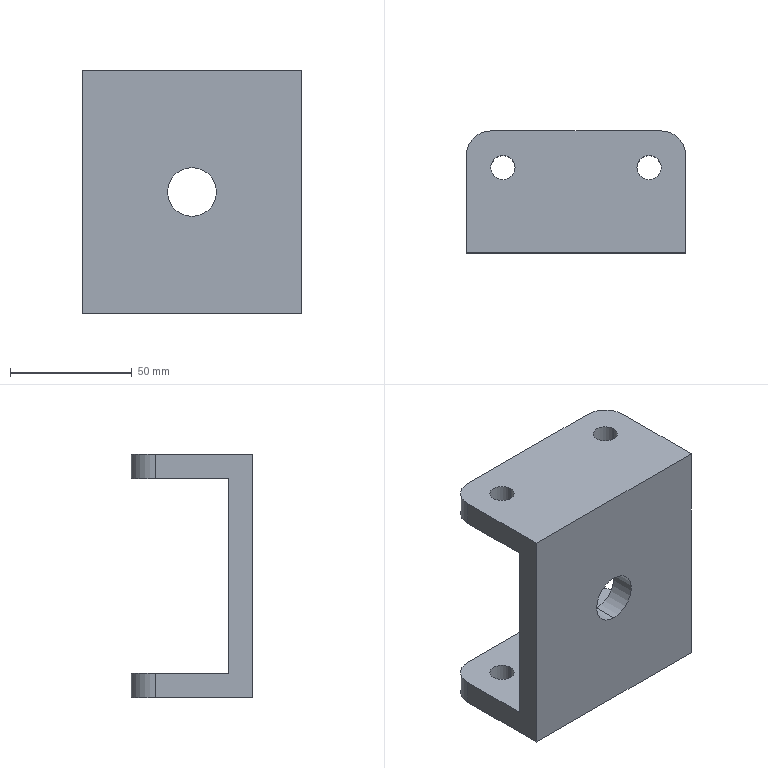Part | SolidWorks | features ICE 4, MoveFace 4, Extrusion 1, Fillet 1 | 1 solid | 24 faces | box 90 x 50 x 100 mm | volume 154858 mm3 | cylinder 14 | plane 10 | commonest cylinder face diameters 10 x8 20 x6
STEP:
#1=CARTESIAN_POINT('',(-5.,0.,-35.));
#2=VERTEX_POINT('',#1);
#3=CARTESIAN_POINT('',(-5.,0.,-15.));
#4=VERTEX_POINT('',#3);
#5=CARTESIAN_POINT('',(-5.,0.,-25.));
#6=DIRECTION('',(0.,1.,0.));
#7=DIRECTION('',(0.,0.,1.));
#8=AXIS2_PLACEMENT_3D('',#5,#6,#7);
#9=CIRCLE('',#8,10.);
#10=EDGE_CURVE('',#2,#4,#9,.T.);
#11=ORIENTED_EDGE('',*,*,#10,.F.);
#12=CARTESIAN_POINT('',(-5.,10.,-35.));
#13=VERTEX_POINT('',#12);
#14=CARTESIAN_POINT('',(-5.,0.,-35.));
#15=DIRECTION('',(0.,1.,0.));
#16=VECTOR('',#15,1000.);
#17=LINE('',#14,#16);
#18=EDGE_CURVE('',#2,#13,#17,.T.);
#19=ORIENTED_EDGE('',*,*,#18,.T.);
#20=CARTESIAN_POINT('',(-5.,10.,-15.));
#21=VERTEX_POINT('',#20);
#22=CARTESIAN_POINT('',(-5.,10.,-25.));
#23=DIRECTION('',(0.,1.,0.));
#24=DIRECTION('',(0.,0.,1.));
#25=AXIS2_PLACEMENT_3D('',#22,#23,#24);
#26=CIRCLE('',#25,10.);
#27=EDGE_CURVE('',#13,#21,#26,.T.);
#28=ORIENTED_EDGE('',*,*,#27,.T.);
#29=CARTESIAN_POINT('',(-5.,0.,-15.));
#30=DIRECTION('',(0.,1.,0.));
#31=VECTOR('',#30,1000.);
#32=LINE('',#29,#31);
#33=EDGE_CURVE('',#4,#21,#32,.T.);
#34=ORIENTED_EDGE('',*,*,#33,.F.);
#35=EDGE_LOOP('',(#11,#19,#28,#34));
#36=FACE_OUTER_BOUND('',#35,.T.);
#37=CARTESIAN_POINT('',(-5.,0.,-25.));
#38=DIRECTION('',(0.,1.,0.));
#39=DIRECTION('',(0.,0.,1.));
#40=AXIS2_PLACEMENT_3D('',#37,#38,#39);
#41=CYLINDRICAL_SURFACE('',#40,10.);
#42=ADVANCED_FACE('',(#36),#41,.F.);
#43=CARTESIAN_POINT('',(20.,35.,-75.));
#44=VERTEX_POINT('',#43);
#45=CARTESIAN_POINT('',(30.,35.,-75.));
#46=VERTEX_POINT('',#45);
#47=CARTESIAN_POINT('',(25.,35.,-75.));
#48=DIRECTION('',(0.,0.,1.));
#49=DIRECTION('',(1.,0.,0.));
#50=AXIS2_PLACEMENT_3D('',#47,#48,#49);
#51=CIRCLE('',#50,5.);
#52=EDGE_CURVE('',#44,#46,#51,.T.);
#53=ORIENTED_EDGE('',*,*,#52,.F.);
#54=CARTESIAN_POINT('',(20.,35.,-65.));
#55=VERTEX_POINT('',#54);
#56=CARTESIAN_POINT('',(20.,35.,-25.));
#57=DIRECTION('',(0.,0.,1.));
#58=VECTOR('',#57,1000.);
#59=LINE('',#56,#58);
#60=EDGE_CURVE('',#44,#55,#59,.T.);
#61=ORIENTED_EDGE('',*,*,#60,.T.);
#62=CARTESIAN_POINT('',(30.,35.,-65.));
#63=VERTEX_POINT('',#62);
#64=CARTESIAN_POINT('',(25.,35.,-65.));
#65=DIRECTION('',(0.,0.,-1.));
#66=DIRECTION('',(0.,1.,0.));
#67=AXIS2_PLACEMENT_3D('',#64,#65,#66);
#68=CIRCLE('',#67,5.);
#69=EDGE_CURVE('',#63,#55,#68,.T.);
#70=ORIENTED_EDGE('',*,*,#69,.F.);
#71=CARTESIAN_POINT('',(30.,35.,-25.));
#72=DIRECTION('',(0.,0.,1.));
#73=VECTOR('',#72,1000.);
#74=LINE('',#71,#73);
#75=EDGE_CURVE('',#46,#63,#74,.T.);
#76=ORIENTED_EDGE('',*,*,#75,.F.);
#77=EDGE_LOOP('',(#53,#61,#70,#76));
#78=FACE_OUTER_BOUND('',#77,.T.);
#79=CARTESIAN_POINT('',(25.,35.,-25.));
#80=DIRECTION('',(0.,0.,1.));
#81=DIRECTION('',(1.,0.,0.));
#82=AXIS2_PLACEMENT_3D('',#79,#80,#81);
#83=CYLINDRICAL_SURFACE('',#82,5.);
#84=ADVANCED_FACE('',(#78),#83,.F.);
#85=CARTESIAN_POINT('',(-40.,35.,-75.));
#86=VERTEX_POINT('',#85);
#87=CARTESIAN_POINT('',(-30.,35.,-75.));
#88=VERTEX_POINT('',#87);
#89=CARTESIAN_POINT('',(-35.,35.,-75.));
#90=DIRECTION('',(0.,0.,1.));
#91=DIRECTION('',(1.,0.,0.));
#92=AXIS2_PLACEMENT_3D('',#89,#90,#91);
#93=CIRCLE('',#92,5.);
#94=EDGE_CURVE('',#86,#88,#93,.T.);
#95=ORIENTED_EDGE('',*,*,#94,.F.);
#96=CARTESIAN_POINT('',(-40.,35.,-65.));
#97=VERTEX_POINT('',#96);
#98=CARTESIAN_POINT('',(-40.,35.,-25.));
#99=DIRECTION('',(0.,0.,1.));
#100=VECTOR('',#99,1000.);
#101=LINE('',#98,#100);
#102=EDGE_CURVE('',#86,#97,#101,.T.);
#103=ORIENTED_EDGE('',*,*,#102,.T.);
#104=CARTESIAN_POINT('',(-30.,35.,-65.));
#105=VERTEX_POINT('',#104);
#106=CARTESIAN_POINT('',(-35.,35.,-65.));
#107=DIRECTION('',(0.,0.,-1.));
#108=DIRECTION('',(0.,1.,0.));
#109=AXIS2_PLACEMENT_3D('',#106,#107,#108);
#110=CIRCLE('',#109,5.);
#111=EDGE_CURVE('',#105,#97,#110,.T.);
#112=ORIENTED_EDGE('',*,*,#111,.F.);
#113=CARTESIAN_POINT('',(-30.,35.,-25.));
#114=DIRECTION('',(0.,0.,1.));
#115=VECTOR('',#114,1000.);
#116=LINE('',#113,#115);
#117=EDGE_CURVE('',#88,#105,#116,.T.);
#118=ORIENTED_EDGE('',*,*,#117,.F.);
#119=EDGE_LOOP('',(#95,#103,#112,#118));
#120=FACE_OUTER_BOUND('',#119,.T.);
#121=CARTESIAN_POINT('',(-35.,35.,-25.));
#122=DIRECTION('',(0.,0.,1.));
#123=DIRECTION('',(1.,0.,0.));
#124=AXIS2_PLACEMENT_3D('',#121,#122,#123);
#125=CYLINDRICAL_SURFACE('',#124,5.);
#126=ADVANCED_FACE('',(#120),#125,.F.);
#127=CARTESIAN_POINT('',(20.,35.,15.));
#128=VERTEX_POINT('',#127);
#129=CARTESIAN_POINT('',(30.,35.,15.));
#130=VERTEX_POINT('',#129);
#131=CARTESIAN_POINT('',(25.,35.,15.));
#132=DIRECTION('',(0.,0.,1.));
#133=DIRECTION('',(0.,-1.,0.));
#134=AXIS2_PLACEMENT_3D('',#131,#132,#133);
#135=CIRCLE('',#134,5.);
#136=EDGE_CURVE('',#128,#130,#135,.T.);
#137=ORIENTED_EDGE('',*,*,#136,.F.);
#138=CARTESIAN_POINT('',(20.,35.,25.));
#139=VERTEX_POINT('',#138);
#140=CARTESIAN_POINT('',(20.,35.,-25.));
#141=DIRECTION('',(0.,0.,1.));
#142=VECTOR('',#141,1000.);
#143=LINE('',#140,#142);
#144=EDGE_CURVE('',#128,#139,#143,.T.);
#145=ORIENTED_EDGE('',*,*,#144,.T.);
#146=CARTESIAN_POINT('',(30.,35.,25.));
#147=VERTEX_POINT('',#146);
#148=CARTESIAN_POINT('',(25.,35.,25.));
#149=DIRECTION('',(0.,0.,1.));
#150=DIRECTION('',(1.,0.,0.));
#151=AXIS2_PLACEMENT_3D('',#148,#149,#150);
#152=CIRCLE('',#151,5.);
#153=EDGE_CURVE('',#139,#147,#152,.T.);
#154=ORIENTED_EDGE('',*,*,#153,.T.);
#155=CARTESIAN_POINT('',(30.,35.,-25.));
#156=DIRECTION('',(0.,0.,1.));
#157=VECTOR('',#156,1000.);
#158=LINE('',#155,#157);
#159=EDGE_CURVE('',#130,#147,#158,.T.);
#160=ORIENTED_EDGE('',*,*,#159,.F.);
#161=EDGE_LOOP('',(#137,#145,#154,#160));
#162=FACE_OUTER_BOUND('',#161,.T.);
#163=CARTESIAN_POINT('',(25.,35.,-25.));
#164=DIRECTION('',(0.,0.,1.));
#165=DIRECTION('',(1.,0.,0.));
#166=AXIS2_PLACEMENT_3D('',#163,#164,#165);
#167=CYLINDRICAL_SURFACE('',#166,5.);
#168=ADVANCED_FACE('',(#162),#167,.F.);
#169=CARTESIAN_POINT('',(-40.,35.,15.));
#170=VERTEX_POINT('',#169);
#171=CARTESIAN_POINT('',(-30.,35.,15.));
#172=VERTEX_POINT('',#171);
#173=CARTESIAN_POINT('',(-35.,35.,15.));
#174=DIRECTION('',(0.,0.,1.));
#175=DIRECTION('',(0.,-1.,0.));
#176=AXIS2_PLACEMENT_3D('',#173,#174,#175);
#177=CIRCLE('',#176,5.);
#178=EDGE_CURVE('',#170,#172,#177,.T.);
#179=ORIENTED_EDGE('',*,*,#178,.F.);
#180=CARTESIAN_POINT('',(-40.,35.,25.));
#181=VERTEX_POINT('',#180);
#182=CARTESIAN_POINT('',(-40.,35.,-25.));
#183=DIRECTION('',(0.,0.,1.));
#184=VECTOR('',#183,1000.);
#185=LINE('',#182,#184);
#186=EDGE_CURVE('',#170,#181,#185,.T.);
#187=ORIENTED_EDGE('',*,*,#186,.T.);
#188=CARTESIAN_POINT('',(-30.,35.,25.));
#189=VERTEX_POINT('',#188);
#190=CARTESIAN_POINT('',(-35.,35.,25.));
#191=DIRECTION('',(0.,0.,1.));
#192=DIRECTION('',(1.,0.,0.));
#193=AXIS2_PLACEMENT_3D('',#190,#191,#192);
#194=CIRCLE('',#193,5.);
#195=EDGE_CURVE('',#181,#189,#194,.T.);
#196=ORIENTED_EDGE('',*,*,#195,.T.);
#197=CARTESIAN_POINT('',(-30.,35.,-25.));
#198=DIRECTION('',(0.,0.,1.));
#199=VECTOR('',#198,1000.);
#200=LINE('',#197,#199);
#201=EDGE_CURVE('',#172,#189,#200,.T.);
#202=ORIENTED_EDGE('',*,*,#201,.F.);
#203=EDGE_LOOP('',(#179,#187,#196,#202));
#204=FACE_OUTER_BOUND('',#203,.T.);
#205=CARTESIAN_POINT('',(-35.,35.,-25.));
#206=DIRECTION('',(0.,0.,1.));
#207=DIRECTION('',(1.,0.,0.));
#208=AXIS2_PLACEMENT_3D('',#205,#206,#207);
#209=CYLINDRICAL_SURFACE('',#208,5.);
#210=ADVANCED_FACE('',(#204),#209,.F.);
#211=CARTESIAN_POINT('',(30.,50.,-65.));
#212=VERTEX_POINT('',#211);
#213=CARTESIAN_POINT('',(-40.,50.,-65.));
#214=VERTEX_POINT('',#213);
#215=CARTESIAN_POINT('',(40.,50.,-65.));
#216=DIRECTION('',(-1.,0.,0.));
#217=VECTOR('',#216,1000.);
#218=LINE('',#215,#217);
#219=EDGE_CURVE('',#212,#214,#218,.T.);
#220=ORIENTED_EDGE('',*,*,#219,.F.);
#221=CARTESIAN_POINT('',(30.,50.,-75.));
#222=VERTEX_POINT('',#221);
#223=CARTESIAN_POINT('',(30.,50.,0.));
#224=DIRECTION('',(0.,0.,-1.));
#225=VECTOR('',#224,1000.);
#226=LINE('',#223,#225);
#227=EDGE_CURVE('',#212,#222,#226,.T.);
#228=ORIENTED_EDGE('',*,*,#227,.T.);
#229=CARTESIAN_POINT('',(-40.,50.,-75.));
#230=VERTEX_POINT('',#229);
#231=CARTESIAN_POINT('',(-40.,50.,-75.));
#232=DIRECTION('',(-1.,0.,0.));
#233=VECTOR('',#232,1000.);
#234=LINE('',#231,#233);
#235=EDGE_CURVE('',#222,#230,#234,.T.);
#236=ORIENTED_EDGE('',*,*,#235,.T.);
#237=CARTESIAN_POINT('',(-40.,50.,0.));
#238=DIRECTION('',(0.,0.,1.));
#239=VECTOR('',#238,1000.);
#240=LINE('',#237,#239);
#241=EDGE_CURVE('',#230,#214,#240,.T.);
#242=ORIENTED_EDGE('',*,*,#241,.T.);
#243=EDGE_LOOP('',(#220,#228,#236,#242));
#244=FACE_OUTER_BOUND('',#243,.T.);
#245=CARTESIAN_POINT('',(0.,50.,0.));
#246=DIRECTION('',(0.,-1.,0.));
#247=DIRECTION('',(0.,0.,-1.));
#248=AXIS2_PLACEMENT_3D('',#245,#246,#247);
#249=PLANE('',#248);
#250=ADVANCED_FACE('',(#244),#249,.F.);
#251=CARTESIAN_POINT('',(40.,40.,-75.));
#252=VERTEX_POINT('',#251);
#253=CARTESIAN_POINT('',(40.,0.,-75.));
#254=VERTEX_POINT('',#253);
#255=CARTESIAN_POINT('',(40.,50.,-75.));
#256=DIRECTION('',(0.,-1.,0.));
#257=VECTOR('',#256,1000.);
#258=LINE('',#255,#257);
#259=EDGE_CURVE('',#252,#254,#258,.T.);
#260=ORIENTED_EDGE('',*,*,#259,.F.);
#261=CARTESIAN_POINT('',(40.,40.,-65.));
#262=VERTEX_POINT('',#261);
#263=CARTESIAN_POINT('',(40.,40.,25.));
#264=DIRECTION('',(0.,0.,1.));
#265=VECTOR('',#264,1000.);
#266=LINE('',#263,#265);
#267=EDGE_CURVE('',#252,#262,#266,.T.);
#268=ORIENTED_EDGE('',*,*,#267,.T.);
#269=CARTESIAN_POINT('',(40.,10.,-65.));
#270=VERTEX_POINT('',#269);
#271=CARTESIAN_POINT('',(40.,50.,-65.));
#272=DIRECTION('',(0.,-1.,0.));
#273=VECTOR('',#272,1000.);
#274=LINE('',#271,#273);
#275=EDGE_CURVE('',#262,#270,#274,.T.);
#276=ORIENTED_EDGE('',*,*,#275,.T.);
#277=CARTESIAN_POINT('',(40.,10.,15.));
#278=VERTEX_POINT('',#277);
#279=CARTESIAN_POINT('',(40.,10.,-15.));
#280=DIRECTION('',(0.,0.,1.));
#281=VECTOR('',#280,1000.);
#282=LINE('',#279,#281);
#283=EDGE_CURVE('',#270,#278,#282,.T.);
#284=ORIENTED_EDGE('',*,*,#283,.T.);
#285=CARTESIAN_POINT('',(40.,40.,15.));
#286=VERTEX_POINT('',#285);
#287=CARTESIAN_POINT('',(40.,50.,15.));
#288=DIRECTION('',(0.,1.,0.));
#289=VECTOR('',#288,1000.);
#290=LINE('',#287,#289);
#291=EDGE_CURVE('',#278,#286,#290,.T.);
#292=ORIENTED_EDGE('',*,*,#291,.T.);
#293=CARTESIAN_POINT('',(40.,40.,25.));
#294=VERTEX_POINT('',#293);
#295=CARTESIAN_POINT('',(40.,40.,25.));
#296=DIRECTION('',(0.,0.,1.));
#297=VECTOR('',#296,1000.);
#298=LINE('',#295,#297);
#299=EDGE_CURVE('',#286,#294,#298,.T.);
#300=ORIENTED_EDGE('',*,*,#299,.T.);
#301=CARTESIAN_POINT('',(40.,0.,25.));
#302=VERTEX_POINT('',#301);
#303=CARTESIAN_POINT('',(40.,50.,25.));
#304=DIRECTION('',(0.,-1.,0.));
#305=VECTOR('',#304,1000.);
#306=LINE('',#303,#305);
#307=EDGE_CURVE('',#294,#302,#306,.T.);
#308=ORIENTED_EDGE('',*,*,#307,.T.);
#309=CARTESIAN_POINT('',(40.,0.,25.));
#310=DIRECTION('',(0.,0.,-1.));
#311=VECTOR('',#310,1000.);
#312=LINE('',#309,#311);
#313=EDGE_CURVE('',#302,#254,#312,.T.);
#314=ORIENTED_EDGE('',*,*,#313,.T.);
#315=EDGE_LOOP('',(#260,#268,#276,#284,#292,#300,#308,#314));
#316=FACE_OUTER_BOUND('',#315,.T.);
#317=CARTESIAN_POINT('',(40.,50.,25.));
#318=DIRECTION('',(-1.,0.,0.));
#319=DIRECTION('',(0.,0.,1.));
#320=AXIS2_PLACEMENT_3D('',#317,#318,#319);
#321=PLANE('',#320);
#322=ADVANCED_FACE('',(#316),#321,.F.);
#323=CARTESIAN_POINT('',(25.,35.,-75.));
#324=DIRECTION('',(0.,0.,1.));
#325=DIRECTION('',(1.,0.,0.));
#326=AXIS2_PLACEMENT_3D('',#323,#324,#325);
#327=CIRCLE('',#326,5.);
#328=EDGE_CURVE('',#46,#44,#327,.T.);
#329=ORIENTED_EDGE('',*,*,#328,.T.);
#330=ORIENTED_EDGE('',*,*,#52,.T.);
#331=EDGE_LOOP('',(#329,#330));
#332=FACE_BOUND('',#331,.T.);
#333=CARTESIAN_POINT('',(-35.,35.,-75.));
#334=DIRECTION('',(0.,0.,1.));
#335=DIRECTION('',(1.,0.,0.));
#336=AXIS2_PLACEMENT_3D('',#333,#334,#335);
#337=CIRCLE('',#336,5.);
#338=EDGE_CURVE('',#88,#86,#337,.T.);
#339=ORIENTED_EDGE('',*,*,#338,.T.);
#340=ORIENTED_EDGE('',*,*,#94,.T.);
#341=EDGE_LOOP('',(#339,#340));
#342=FACE_BOUND('',#341,.T.);
#343=ORIENTED_EDGE('',*,*,#235,.F.);
#344=CARTESIAN_POINT('',(30.,40.,-75.));
#345=DIRECTION('',(0.,0.,-1.));
#346=DIRECTION('',(1.,0.,0.));
#347=AXIS2_PLACEMENT_3D('',#344,#345,#346);
#348=CIRCLE('',#347,10.);
#349=EDGE_CURVE('',#222,#252,#348,.T.);
#350=ORIENTED_EDGE('',*,*,#349,.T.);
#351=ORIENTED_EDGE('',*,*,#259,.T.);
#352=CARTESIAN_POINT('',(-50.,0.,-75.));
#353=VERTEX_POINT('',#352);
#354=CARTESIAN_POINT('',(-40.,0.,-75.));
#355=DIRECTION('',(-1.,0.,0.));
#356=VECTOR('',#355,1000.);
#357=LINE('',#354,#356);
#358=EDGE_CURVE('',#254,#353,#357,.T.);
#359=ORIENTED_EDGE('',*,*,#358,.T.);
#360=CARTESIAN_POINT('',(-50.,40.,-75.));
#361=VERTEX_POINT('',#360);
#362=CARTESIAN_POINT('',(-50.,50.,-75.));
#363=DIRECTION('',(0.,-1.,0.));
#364=VECTOR('',#363,1000.);
#365=LINE('',#362,#364);
#366=EDGE_CURVE('',#361,#353,#365,.T.);
#367=ORIENTED_EDGE('',*,*,#366,.F.);
#368=CARTESIAN_POINT('',(-40.,40.,-75.));
#369=DIRECTION('',(0.,0.,-1.));
#370=DIRECTION('',(1.,0.,0.));
#371=AXIS2_PLACEMENT_3D('',#368,#369,#370);
#372=CIRCLE('',#371,10.);
#373=EDGE_CURVE('',#361,#230,#372,.T.);
#374=ORIENTED_EDGE('',*,*,#373,.T.);
#375=EDGE_LOOP('',(#343,#350,#351,#359,#367,#374));
#376=FACE_OUTER_BOUND('',#375,.T.);
#377=CARTESIAN_POINT('',(-40.,50.,-75.));
#378=DIRECTION('',(0.,0.,1.));
#379=DIRECTION('',(1.,0.,0.));
#380=AXIS2_PLACEMENT_3D('',#377,#378,#379);
#381=PLANE('',#380);
#382=ADVANCED_FACE('',(#332,#342,#376),#381,.F.);
#383=CARTESIAN_POINT('',(-50.,40.,25.));
#384=VERTEX_POINT('',#383);
#385=CARTESIAN_POINT('',(-50.,0.,25.));
#386=VERTEX_POINT('',#385);
#387=CARTESIAN_POINT('',(-50.,50.,25.));
#388=DIRECTION('',(0.,-1.,0.));
#389=VECTOR('',#388,1000.);
#390=LINE('',#387,#389);
#391=EDGE_CURVE('',#384,#386,#390,.T.);
#392=ORIENTED_EDGE('',*,*,#391,.F.);
#393=CARTESIAN_POINT('',(-50.,40.,15.));
#394=VERTEX_POINT('',#393);
#395=CARTESIAN_POINT('',(-50.,40.,25.));
#396=DIRECTION('',(0.,0.,-1.));
#397=VECTOR('',#396,1000.);
#398=LINE('',#395,#397);
#399=EDGE_CURVE('',#384,#394,#398,.T.);
#400=ORIENTED_EDGE('',*,*,#399,.T.);
#401=CARTESIAN_POINT('',(-50.,10.,15.));
#402=VERTEX_POINT('',#401);
#403=CARTESIAN_POINT('',(-50.,50.,15.));
#404=DIRECTION('',(0.,1.,0.));
#405=VECTOR('',#404,1000.);
#406=LINE('',#403,#405);
#407=EDGE_CURVE('',#402,#394,#406,.T.);
#408=ORIENTED_EDGE('',*,*,#407,.F.);
#409=CARTESIAN_POINT('',(-50.,10.,-65.));
#410=VERTEX_POINT('',#409);
#411=CARTESIAN_POINT('',(-50.,10.,-15.));
#412=DIRECTION('',(0.,0.,1.));
#413=VECTOR('',#412,1000.);
#414=LINE('',#411,#413);
#415=EDGE_CURVE('',#410,#402,#414,.T.);
#416=ORIENTED_EDGE('',*,*,#415,.F.);
#417=CARTESIAN_POINT('',(-50.,40.,-65.));
#418=VERTEX_POINT('',#417);
#419=CARTESIAN_POINT('',(-50.,50.,-65.));
#420=DIRECTION('',(0.,-1.,0.));
#421=VECTOR('',#420,1000.);
#422=LINE('',#419,#421);
#423=EDGE_CURVE('',#418,#410,#422,.T.);
#424=ORIENTED_EDGE('',*,*,#423,.F.);
#425=CARTESIAN_POINT('',(-50.,40.,25.));
#426=DIRECTION('',(0.,0.,-1.));
#427=VECTOR('',#426,1000.);
#428=LINE('',#425,#427);
#429=EDGE_CURVE('',#418,#361,#428,.T.);
#430=ORIENTED_EDGE('',*,*,#429,.T.);
#431=ORIENTED_EDGE('',*,*,#366,.T.);
#432=CARTESIAN_POINT('',(-50.,0.,25.));
#433=DIRECTION('',(0.,0.,1.));
#434=VECTOR('',#433,1000.);
#435=LINE('',#432,#434);
#436=EDGE_CURVE('',#353,#386,#435,.T.);
#437=ORIENTED_EDGE('',*,*,#436,.T.);
#438=EDGE_LOOP('',(#392,#400,#408,#416,#424,#430,#431,#437));
#439=FACE_OUTER_BOUND('',#438,.T.);
#440=CARTESIAN_POINT('',(-50.,50.,25.));
#441=DIRECTION('',(1.,0.,0.));
#442=DIRECTION('',(0.,0.,-1.));
#443=AXIS2_PLACEMENT_3D('',#440,#441,#442);
#444=PLANE('',#443);
#445=ADVANCED_FACE('',(#439),#444,.F.);
#446=CARTESIAN_POINT('',(25.,35.,25.));
#447=DIRECTION('',(0.,0.,1.));
#448=DIRECTION('',(1.,0.,0.));
#449=AXIS2_PLACEMENT_3D('',#446,#447,#448);
#450=CIRCLE('',#449,5.);
#451=EDGE_CURVE('',#147,#139,#450,.T.);
#452=ORIENTED_EDGE('',*,*,#451,.F.);
#453=ORIENTED_EDGE('',*,*,#153,.F.);
#454=EDGE_LOOP('',(#452,#453));
#455=FACE_BOUND('',#454,.T.);
#456=CARTESIAN_POINT('',(-35.,35.,25.));
#457=DIRECTION('',(0.,0.,1.));
#458=DIRECTION('',(1.,0.,0.));
#459=AXIS2_PLACEMENT_3D('',#456,#457,#458);
#460=CIRCLE('',#459,5.);
#461=EDGE_CURVE('',#189,#181,#460,.T.);
#462=ORIENTED_EDGE('',*,*,#461,.F.);
#463=ORIENTED_EDGE('',*,*,#195,.F.);
#464=EDGE_LOOP('',(#462,#463));
#465=FACE_BOUND('',#464,.T.);
#466=ORIENTED_EDGE('',*,*,#307,.F.);
#467=CARTESIAN_POINT('',(30.,50.,25.));
#468=VERTEX_POINT('',#467);
#469=CARTESIAN_POINT('',(30.,40.,25.));
#470=DIRECTION('',(0.,0.,1.));
#471=DIRECTION('',(-1.,0.,0.));
#472=AXIS2_PLACEMENT_3D('',#469,#470,#471);
#473=CIRCLE('',#472,10.);
#474=EDGE_CURVE('',#294,#468,#473,.T.);
#475=ORIENTED_EDGE('',*,*,#474,.T.);
#476=CARTESIAN_POINT('',(-40.,50.,25.));
#477=VERTEX_POINT('',#476);
#478=CARTESIAN_POINT('',(-40.,50.,25.));
#479=DIRECTION('',(1.,0.,0.));
#480=VECTOR('',#479,1000.);
#481=LINE('',#478,#480);
#482=EDGE_CURVE('',#477,#468,#481,.T.);
#483=ORIENTED_EDGE('',*,*,#482,.F.);
#484=CARTESIAN_POINT('',(-40.,40.,25.));
#485=DIRECTION('',(0.,0.,1.));
#486=DIRECTION('',(-1.,0.,0.));
#487=AXIS2_PLACEMENT_3D('',#484,#485,#486);
#488=CIRCLE('',#487,10.);
#489=EDGE_CURVE('',#477,#384,#488,.T.);
#490=ORIENTED_EDGE('',*,*,#489,.T.);
#491=ORIENTED_EDGE('',*,*,#391,.T.);
#492=CARTESIAN_POINT('',(-40.,0.,25.));
#493=DIRECTION('',(1.,0.,0.));
#494=VECTOR('',#493,1000.);
#495=LINE('',#492,#494);
#496=EDGE_CURVE('',#386,#302,#495,.T.);
#497=ORIENTED_EDGE('',*,*,#496,.T.);
#498=EDGE_LOOP('',(#466,#475,#483,#490,#491,#497));
#499=FACE_OUTER_BOUND('',#498,.T.);
#500=CARTESIAN_POINT('',(-40.,50.,25.));
#501=DIRECTION('',(0.,0.,-1.));
#502=DIRECTION('',(-1.,0.,0.));
#503=AXIS2_PLACEMENT_3D('',#500,#501,#502);
#504=PLANE('',#503);
#505=ADVANCED_FACE('',(#455,#465,#499),#504,.F.);
#506=ORIENTED_EDGE('',*,*,#482,.T.);
#507=CARTESIAN_POINT('',(30.,50.,15.));
#508=VERTEX_POINT('',#507);
#509=CARTESIAN_POINT('',(30.,50.,0.));
#510=DIRECTION('',(0.,0.,-1.));
#511=VECTOR('',#510,1000.);
#512=LINE('',#509,#511);
#513=EDGE_CURVE('',#468,#508,#512,.T.);
#514=ORIENTED_EDGE('',*,*,#513,.T.);
#515=CARTESIAN_POINT('',(-40.,50.,15.));
#516=VERTEX_POINT('',#515);
#517=CARTESIAN_POINT('',(40.,50.,15.));
#518=DIRECTION('',(-1.,0.,0.));
#519=VECTOR('',#518,1000.);
#520=LINE('',#517,#519);
#521=EDGE_CURVE('',#508,#516,#520,.T.);
#522=ORIENTED_EDGE('',*,*,#521,.T.);
#523=CARTESIAN_POINT('',(-40.,50.,0.));
#524=DIRECTION('',(0.,0.,1.));
#525=VECTOR('',#524,1000.);
#526=LINE('',#523,#525);
#527=EDGE_CURVE('',#516,#477,#526,.T.);
#528=ORIENTED_EDGE('',*,*,#527,.T.);
#529=EDGE_LOOP('',(#506,#514,#522,#528));
#530=FACE_OUTER_BOUND('',#529,.T.);
#531=CARTESIAN_POINT('',(0.,50.,0.));
#532=DIRECTION('',(0.,-1.,0.));
#533=DIRECTION('',(0.,0.,-1.));
#534=AXIS2_PLACEMENT_3D('',#531,#532,#533);
#535=PLANE('',#534);
#536=ADVANCED_FACE('',(#530),#535,.F.);
#537=CARTESIAN_POINT('',(-5.,0.,-25.));
#538=DIRECTION('',(0.,1.,0.));
#539=DIRECTION('',(0.,0.,1.));
#540=AXIS2_PLACEMENT_3D('',#537,#538,#539);
#541=CIRCLE('',#540,10.);
#542=EDGE_CURVE('',#4,#2,#541,.T.);
#543=ORIENTED_EDGE('',*,*,#542,.T.);
#544=ORIENTED_EDGE('',*,*,#10,.T.);
#545=EDGE_LOOP('',(#543,#544));
#546=FACE_BOUND('',#545,.T.);
#547=ORIENTED_EDGE('',*,*,#313,.F.);
#548=ORIENTED_EDGE('',*,*,#496,.F.);
#549=ORIENTED_EDGE('',*,*,#436,.F.);
#550=ORIENTED_EDGE('',*,*,#358,.F.);
#551=EDGE_LOOP('',(#547,#548,#549,#550));
#552=FACE_OUTER_BOUND('',#551,.T.);
#553=CARTESIAN_POINT('',(0.,0.,0.));
#554=DIRECTION('',(0.,-1.,0.));
#555=DIRECTION('',(0.,0.,-1.));
#556=AXIS2_PLACEMENT_3D('',#553,#554,#555);
#557=PLANE('',#556);
#558=ADVANCED_FACE('',(#546,#552),#557,.T.);
#559=ORIENTED_EDGE('',*,*,#69,.T.);
#560=CARTESIAN_POINT('',(25.,35.,-65.));
#561=DIRECTION('',(0.,0.,-1.));
#562=DIRECTION('',(0.,1.,0.));
#563=AXIS2_PLACEMENT_3D('',#560,#561,#562);
#564=CIRCLE('',#563,5.);
#565=EDGE_CURVE('',#55,#63,#564,.T.);
#566=ORIENTED_EDGE('',*,*,#565,.T.);
#567=EDGE_LOOP('',(#559,#566));
#568=FACE_BOUND('',#567,.T.);
#569=ORIENTED_EDGE('',*,*,#111,.T.);
#570=CARTESIAN_POINT('',(-35.,35.,-65.));
#571=DIRECTION('',(0.,0.,-1.));
#572=DIRECTION('',(0.,1.,0.));
#573=AXIS2_PLACEMENT_3D('',#570,#571,#572);
#574=CIRCLE('',#573,5.);
#575=EDGE_CURVE('',#97,#105,#574,.T.);
#576=ORIENTED_EDGE('',*,*,#575,.T.);
#577=EDGE_LOOP('',(#569,#576));
#578=FACE_BOUND('',#577,.T.);
#579=ORIENTED_EDGE('',*,*,#275,.F.);
#580=CARTESIAN_POINT('',(30.,40.,-65.));
#581=DIRECTION('',(0.,0.,1.));
#582=DIRECTION('',(0.,1.,0.));
#583=AXIS2_PLACEMENT_3D('',#580,#581,#582);
#584=CIRCLE('',#583,10.);
#585=EDGE_CURVE('',#262,#212,#584,.T.);
#586=ORIENTED_EDGE('',*,*,#585,.T.);
#587=ORIENTED_EDGE('',*,*,#219,.T.);
#588=CARTESIAN_POINT('',(-40.,40.,-65.));
#589=DIRECTION('',(0.,0.,1.));
#590=DIRECTION('',(0.,1.,0.));
#591=AXIS2_PLACEMENT_3D('',#588,#589,#590);
#592=CIRCLE('',#591,10.);
#593=EDGE_CURVE('',#214,#418,#592,.T.);
#594=ORIENTED_EDGE('',*,*,#593,.T.);
#595=ORIENTED_EDGE('',*,*,#423,.T.);
#596=CARTESIAN_POINT('',(40.,10.,-65.));
#597=DIRECTION('',(-1.,0.,0.));
#598=VECTOR('',#597,1000.);
#599=LINE('',#596,#598);
#600=EDGE_CURVE('',#270,#410,#599,.T.);
#601=ORIENTED_EDGE('',*,*,#600,.F.);
#602=EDGE_LOOP('',(#579,#586,#587,#594,#595,#601));
#603=FACE_OUTER_BOUND('',#602,.T.);
#604=CARTESIAN_POINT('',(40.,50.,-65.));
#605=DIRECTION('',(0.,0.,-1.));
#606=DIRECTION('',(0.,1.,0.));
#607=AXIS2_PLACEMENT_3D('',#604,#605,#606);
#608=PLANE('',#607);
#609=ADVANCED_FACE('',(#568,#578,#603),#608,.F.);
#610=CARTESIAN_POINT('',(25.,35.,15.));
#611=DIRECTION('',(0.,0.,1.));
#612=DIRECTION('',(0.,-1.,0.));
#613=AXIS2_PLACEMENT_3D('',#610,#611,#612);
#614=CIRCLE('',#613,5.);
#615=EDGE_CURVE('',#130,#128,#614,.T.);
#616=ORIENTED_EDGE('',*,*,#615,.T.);
#617=ORIENTED_EDGE('',*,*,#136,.T.);
#618=EDGE_LOOP('',(#616,#617));
#619=FACE_BOUND('',#618,.T.);
#620=CARTESIAN_POINT('',(-35.,35.,15.));
#621=DIRECTION('',(0.,0.,1.));
#622=DIRECTION('',(0.,-1.,0.));
#623=AXIS2_PLACEMENT_3D('',#620,#621,#622);
#624=CIRCLE('',#623,5.);
#625=EDGE_CURVE('',#172,#170,#624,.T.);
#626=ORIENTED_EDGE('',*,*,#625,.T.);
#627=ORIENTED_EDGE('',*,*,#178,.T.);
#628=EDGE_LOOP('',(#626,#627));
#629=FACE_BOUND('',#628,.T.);
#630=ORIENTED_EDGE('',*,*,#521,.F.);
#631=CARTESIAN_POINT('',(30.,40.,15.));
#632=DIRECTION('',(0.,0.,-1.));
#633=DIRECTION('',(0.,-1.,0.));
#634=AXIS2_PLACEMENT_3D('',#631,#632,#633);
#635=CIRCLE('',#634,10.);
#636=EDGE_CURVE('',#508,#286,#635,.T.);
#637=ORIENTED_EDGE('',*,*,#636,.T.);
#638=ORIENTED_EDGE('',*,*,#291,.F.);
#639=CARTESIAN_POINT('',(40.,10.,15.));
#640=DIRECTION('',(-1.,0.,0.));
#641=VECTOR('',#640,1000.);
#642=LINE('',#639,#641);
#643=EDGE_CURVE('',#278,#402,#642,.T.);
#644=ORIENTED_EDGE('',*,*,#643,.T.);
#645=ORIENTED_EDGE('',*,*,#407,.T.);
#646=CARTESIAN_POINT('',(-40.,40.,15.));
#647=DIRECTION('',(0.,0.,-1.));
#648=DIRECTION('',(0.,-1.,0.));
#649=AXIS2_PLACEMENT_3D('',#646,#647,#648);
#650=CIRCLE('',#649,10.);
#651=EDGE_CURVE('',#394,#516,#650,.T.);
#652=ORIENTED_EDGE('',*,*,#651,.T.);
#653=EDGE_LOOP('',(#630,#637,#638,#644,#645,#652));
#654=FACE_OUTER_BOUND('',#653,.T.);
#655=CARTESIAN_POINT('',(40.,50.,15.));
#656=DIRECTION('',(0.,0.,1.));
#657=DIRECTION('',(0.,-1.,0.));
#658=AXIS2_PLACEMENT_3D('',#655,#656,#657);
#659=PLANE('',#658);
#660=ADVANCED_FACE('',(#619,#629,#654),#659,.F.);
#661=CARTESIAN_POINT('',(-5.,10.,-25.));
#662=DIRECTION('',(0.,1.,0.));
#663=DIRECTION('',(0.,0.,1.));
#664=AXIS2_PLACEMENT_3D('',#661,#662,#663);
#665=CIRCLE('',#664,10.);
#666=EDGE_CURVE('',#21,#13,#665,.T.);
#667=ORIENTED_EDGE('',*,*,#666,.F.);
#668=ORIENTED_EDGE('',*,*,#27,.F.);
#669=EDGE_LOOP('',(#667,#668));
#670=FACE_BOUND('',#669,.T.);
#671=ORIENTED_EDGE('',*,*,#415,.T.);
#672=ORIENTED_EDGE('',*,*,#643,.F.);
#673=ORIENTED_EDGE('',*,*,#283,.F.);
#674=ORIENTED_EDGE('',*,*,#600,.T.);
#675=EDGE_LOOP('',(#671,#672,#673,#674));
#676=FACE_OUTER_BOUND('',#675,.T.);
#677=CARTESIAN_POINT('',(40.,10.,-15.));
#678=DIRECTION('',(0.,-1.,0.));
#679=DIRECTION('',(0.,0.,-1.));
#680=AXIS2_PLACEMENT_3D('',#677,#678,#679);
#681=PLANE('',#680);
#682=ADVANCED_FACE('',(#670,#676),#681,.F.);
#683=ORIENTED_EDGE('',*,*,#585,.F.);
#684=ORIENTED_EDGE('',*,*,#267,.F.);
#685=ORIENTED_EDGE('',*,*,#349,.F.);
#686=ORIENTED_EDGE('',*,*,#227,.F.);
#687=EDGE_LOOP('',(#683,#684,#685,#686));
#688=FACE_OUTER_BOUND('',#687,.T.);
#689=CARTESIAN_POINT('',(30.,40.,0.));
#690=DIRECTION('',(0.,0.,-1.));
#691=DIRECTION('',(-1.,0.,0.));
#692=AXIS2_PLACEMENT_3D('',#689,#690,#691);
#693=CYLINDRICAL_SURFACE('',#692,10.);
#694=ADVANCED_FACE('',(#688),#693,.T.);
#695=ORIENTED_EDGE('',*,*,#474,.F.);
#696=ORIENTED_EDGE('',*,*,#299,.F.);
#697=ORIENTED_EDGE('',*,*,#636,.F.);
#698=ORIENTED_EDGE('',*,*,#513,.F.);
#699=EDGE_LOOP('',(#695,#696,#697,#698));
#700=FACE_OUTER_BOUND('',#699,.T.);
#701=CARTESIAN_POINT('',(30.,40.,0.));
#702=DIRECTION('',(0.,0.,-1.));
#703=DIRECTION('',(-1.,0.,0.));
#704=AXIS2_PLACEMENT_3D('',#701,#702,#703);
#705=CYLINDRICAL_SURFACE('',#704,10.);
#706=ADVANCED_FACE('',(#700),#705,.T.);
#707=ORIENTED_EDGE('',*,*,#651,.F.);
#708=ORIENTED_EDGE('',*,*,#399,.F.);
#709=ORIENTED_EDGE('',*,*,#489,.F.);
#710=ORIENTED_EDGE('',*,*,#527,.F.);
#711=EDGE_LOOP('',(#707,#708,#709,#710));
#712=FACE_OUTER_BOUND('',#711,.T.);
#713=CARTESIAN_POINT('',(-40.,40.,0.));
#714=DIRECTION('',(0.,0.,1.));
#715=DIRECTION('',(1.,0.,0.));
#716=AXIS2_PLACEMENT_3D('',#713,#714,#715);
#717=CYLINDRICAL_SURFACE('',#716,10.);
#718=ADVANCED_FACE('',(#712),#717,.T.);
#719=ORIENTED_EDGE('',*,*,#373,.F.);
#720=ORIENTED_EDGE('',*,*,#429,.F.);
#721=ORIENTED_EDGE('',*,*,#593,.F.);
#722=ORIENTED_EDGE('',*,*,#241,.F.);
#723=EDGE_LOOP('',(#719,#720,#721,#722));
#724=FACE_OUTER_BOUND('',#723,.T.);
#725=CARTESIAN_POINT('',(-40.,40.,0.));
#726=DIRECTION('',(0.,0.,1.));
#727=DIRECTION('',(1.,0.,0.));
#728=AXIS2_PLACEMENT_3D('',#725,#726,#727);
#729=CYLINDRICAL_SURFACE('',#728,10.);
#730=ADVANCED_FACE('',(#724),#729,.T.);
#731=ORIENTED_EDGE('',*,*,#186,.F.);
#732=ORIENTED_EDGE('',*,*,#625,.F.);
#733=ORIENTED_EDGE('',*,*,#201,.T.);
#734=ORIENTED_EDGE('',*,*,#461,.T.);
#735=EDGE_LOOP('',(#731,#732,#733,#734));
#736=FACE_OUTER_BOUND('',#735,.T.);
#737=CARTESIAN_POINT('',(-35.,35.,-25.));
#738=DIRECTION('',(0.,0.,1.));
#739=DIRECTION('',(1.,0.,0.));
#740=AXIS2_PLACEMENT_3D('',#737,#738,#739);
#741=CYLINDRICAL_SURFACE('',#740,5.);
#742=ADVANCED_FACE('',(#736),#741,.F.);
#743=ORIENTED_EDGE('',*,*,#144,.F.);
#744=ORIENTED_EDGE('',*,*,#615,.F.);
#745=ORIENTED_EDGE('',*,*,#159,.T.);
#746=ORIENTED_EDGE('',*,*,#451,.T.);
#747=EDGE_LOOP('',(#743,#744,#745,#746));
#748=FACE_OUTER_BOUND('',#747,.T.);
#749=CARTESIAN_POINT('',(25.,35.,-25.));
#750=DIRECTION('',(0.,0.,1.));
#751=DIRECTION('',(1.,0.,0.));
#752=AXIS2_PLACEMENT_3D('',#749,#750,#751);
#753=CYLINDRICAL_SURFACE('',#752,5.);
#754=ADVANCED_FACE('',(#748),#753,.F.);
#755=ORIENTED_EDGE('',*,*,#102,.F.);
#756=ORIENTED_EDGE('',*,*,#338,.F.);
#757=ORIENTED_EDGE('',*,*,#117,.T.);
#758=ORIENTED_EDGE('',*,*,#575,.F.);
#759=EDGE_LOOP('',(#755,#756,#757,#758));
#760=FACE_OUTER_BOUND('',#759,.T.);
#761=CARTESIAN_POINT('',(-35.,35.,-25.));
#762=DIRECTION('',(0.,0.,1.));
#763=DIRECTION('',(1.,0.,0.));
#764=AXIS2_PLACEMENT_3D('',#761,#762,#763);
#765=CYLINDRICAL_SURFACE('',#764,5.);
#766=ADVANCED_FACE('',(#760),#765,.F.);
#767=ORIENTED_EDGE('',*,*,#60,.F.);
#768=ORIENTED_EDGE('',*,*,#328,.F.);
#769=ORIENTED_EDGE('',*,*,#75,.T.);
#770=ORIENTED_EDGE('',*,*,#565,.F.);
#771=EDGE_LOOP('',(#767,#768,#769,#770));
#772=FACE_OUTER_BOUND('',#771,.T.);
#773=CARTESIAN_POINT('',(25.,35.,-25.));
#774=DIRECTION('',(0.,0.,1.));
#775=DIRECTION('',(1.,0.,0.));
#776=AXIS2_PLACEMENT_3D('',#773,#774,#775);
#777=CYLINDRICAL_SURFACE('',#776,5.);
#778=ADVANCED_FACE('',(#772),#777,.F.);
#779=ORIENTED_EDGE('',*,*,#18,.F.);
#780=ORIENTED_EDGE('',*,*,#542,.F.);
#781=ORIENTED_EDGE('',*,*,#33,.T.);
#782=ORIENTED_EDGE('',*,*,#666,.T.);
#783=EDGE_LOOP('',(#779,#780,#781,#782));
#784=FACE_OUTER_BOUND('',#783,.T.);
#785=CARTESIAN_POINT('',(-5.,0.,-25.));
#786=DIRECTION('',(0.,1.,0.));
#787=DIRECTION('',(0.,0.,1.));
#788=AXIS2_PLACEMENT_3D('',#785,#786,#787);
#789=CYLINDRICAL_SURFACE('',#788,10.);
#790=ADVANCED_FACE('',(#784),#789,.F.);
#791=CLOSED_SHELL('',(#42,#84,#126,#168,#210,#250,#322,#382,#445,#505,#536,#558,#609,#660,#682,#694,#706,#718,#730,#742,#754,#766,#778,#790));
#792=MANIFOLD_SOLID_BREP('',#791);
#793=CARTESIAN_POINT('',(0.,0.,0.));
#794=DIRECTION('',(0.,0.,1.));
#795=DIRECTION('',(1.,0.,0.));
#796=AXIS2_PLACEMENT_3D('',#793,#794,#795);
#797=(LENGTH_UNIT()NAMED_UNIT(*)SI_UNIT(.MILLI.,.METRE.));
#798=UNCERTAINTY_MEASURE_WITH_UNIT(LENGTH_MEASURE(0.00001),#797,'','');
#799=(NAMED_UNIT(*)PLANE_ANGLE_UNIT()SI_UNIT($,.RADIAN.));
#800=(NAMED_UNIT(*)SI_UNIT($,.STERADIAN.)SOLID_ANGLE_UNIT());
#801=(GEOMETRIC_REPRESENTATION_CONTEXT(3)GLOBAL_UNCERTAINTY_ASSIGNED_CONTEXT((#798))GLOBAL_UNIT_ASSIGNED_CONTEXT((#797,#799,#800))REPRESENTATION_CONTEXT('',''));
#802=ADVANCED_BREP_SHAPE_REPRESENTATION('',(#792,#796),#801);